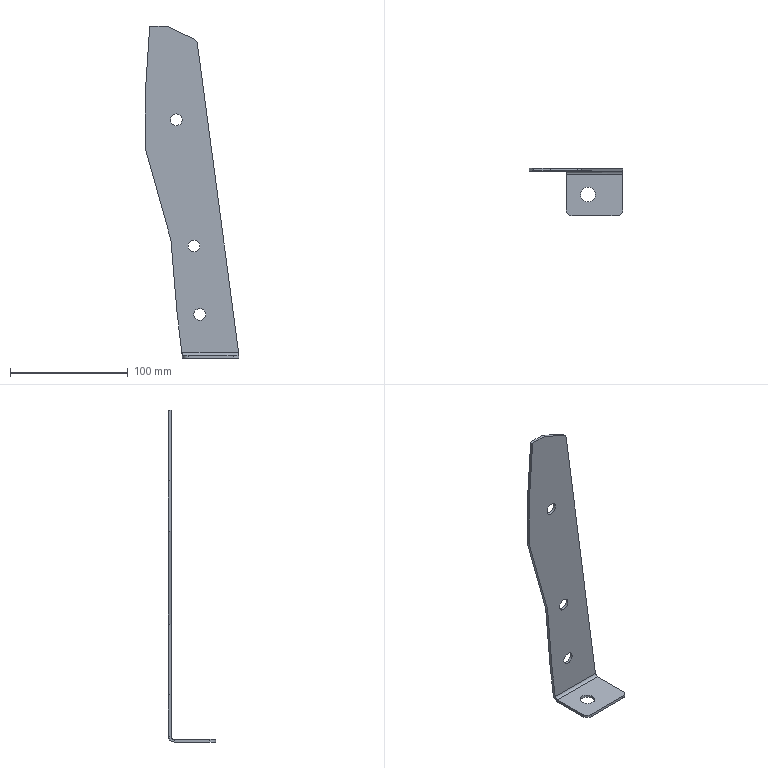Part | SolidWorks | features ICE 2, Fillet 1, FlatPattern 1, SMBaseFlange 1, SheetMetal 1 | 1 solid | 30 faces | box 79.693 x 40 x 281.5 mm | volume 34078 mm3 | plane 15 | cylinder 13 | spline 2 | commonest cylinder face diameters 10 x9 12.5 x2 5 x1 9.6 x1
STEP:
#1=CARTESIAN_POINT('',(3.75,-22.,-279.2));
#2=VERTEX_POINT('',#1);
#3=CARTESIAN_POINT('',(16.25,-22.,-279.2));
#4=VERTEX_POINT('',#3);
#5=CARTESIAN_POINT('',(10.,-22.,-279.2));
#6=DIRECTION('',(0.,0.,1.));
#7=DIRECTION('',(-1.,0.,0.));
#8=AXIS2_PLACEMENT_3D('',#5,#6,#7);
#9=CIRCLE('',#8,6.25);
#10=EDGE_CURVE('',#2,#4,#9,.T.);
#11=ORIENTED_EDGE('',*,*,#10,.T.);
#12=CARTESIAN_POINT('',(16.25,-22.,-281.5));
#13=VERTEX_POINT('',#12);
#14=CARTESIAN_POINT('',(16.25,-22.,0.001));
#15=DIRECTION('',(0.,0.,-1.));
#16=VECTOR('',#15,1000.);
#17=LINE('',#14,#16);
#18=EDGE_CURVE('',#4,#13,#17,.T.);
#19=ORIENTED_EDGE('',*,*,#18,.T.);
#20=CARTESIAN_POINT('',(3.75,-22.,-281.5));
#21=VERTEX_POINT('',#20);
#22=CARTESIAN_POINT('',(10.,-22.,-281.5));
#23=DIRECTION('',(0.,0.,-1.));
#24=DIRECTION('',(-1.,0.,0.));
#25=AXIS2_PLACEMENT_3D('',#22,#23,#24);
#26=CIRCLE('',#25,6.25);
#27=EDGE_CURVE('',#13,#21,#26,.T.);
#28=ORIENTED_EDGE('',*,*,#27,.T.);
#29=CARTESIAN_POINT('',(3.75,-22.,0.001));
#30=DIRECTION('',(0.,0.,-1.));
#31=VECTOR('',#30,1000.);
#32=LINE('',#29,#31);
#33=EDGE_CURVE('',#2,#21,#32,.T.);
#34=ORIENTED_EDGE('',*,*,#33,.F.);
#35=EDGE_LOOP('',(#11,#19,#28,#34));
#36=FACE_OUTER_BOUND('',#35,.T.);
#37=CARTESIAN_POINT('',(10.,-22.,0.001));
#38=DIRECTION('',(0.,0.,-1.));
#39=DIRECTION('',(-1.,0.,0.));
#40=AXIS2_PLACEMENT_3D('',#37,#38,#39);
#41=CYLINDRICAL_SURFACE('',#40,6.25);
#42=ADVANCED_FACE('',(#36),#41,.F.);
#43=CARTESIAN_POINT('',(1.5,-2.3,-191.5));
#44=VERTEX_POINT('',#43);
#45=CARTESIAN_POINT('',(1.5,-2.3,-181.5));
#46=VERTEX_POINT('',#45);
#47=CARTESIAN_POINT('',(1.5,-2.3,-186.5));
#48=DIRECTION('',(0.,1.,0.));
#49=DIRECTION('',(0.,0.,1.));
#50=AXIS2_PLACEMENT_3D('',#47,#48,#49);
#51=CIRCLE('',#50,5.);
#52=EDGE_CURVE('',#44,#46,#51,.T.);
#53=ORIENTED_EDGE('',*,*,#52,.F.);
#54=CARTESIAN_POINT('',(1.5,0.,-191.5));
#55=VERTEX_POINT('',#54);
#56=CARTESIAN_POINT('',(1.5,0.,-191.5));
#57=DIRECTION('',(0.,1.,0.));
#58=VECTOR('',#57,1000.);
#59=LINE('',#56,#58);
#60=EDGE_CURVE('',#44,#55,#59,.T.);
#61=ORIENTED_EDGE('',*,*,#60,.T.);
#62=CARTESIAN_POINT('',(1.5,0.,-181.5));
#63=VERTEX_POINT('',#62);
#64=CARTESIAN_POINT('',(1.5,0.,-186.5));
#65=DIRECTION('',(0.,1.,0.));
#66=DIRECTION('',(0.,0.,1.));
#67=AXIS2_PLACEMENT_3D('',#64,#65,#66);
#68=CIRCLE('',#67,5.);
#69=EDGE_CURVE('',#55,#63,#68,.T.);
#70=ORIENTED_EDGE('',*,*,#69,.T.);
#71=CARTESIAN_POINT('',(1.5,0.,-181.5));
#72=DIRECTION('',(0.,1.,0.));
#73=VECTOR('',#72,1000.);
#74=LINE('',#71,#73);
#75=EDGE_CURVE('',#46,#63,#74,.T.);
#76=ORIENTED_EDGE('',*,*,#75,.F.);
#77=EDGE_LOOP('',(#53,#61,#70,#76));
#78=FACE_OUTER_BOUND('',#77,.T.);
#79=CARTESIAN_POINT('',(1.5,0.,-186.5));
#80=DIRECTION('',(0.,1.,0.));
#81=DIRECTION('',(0.,0.,1.));
#82=AXIS2_PLACEMENT_3D('',#79,#80,#81);
#83=CYLINDRICAL_SURFACE('',#82,5.);
#84=ADVANCED_FACE('',(#78),#83,.F.);
#85=CARTESIAN_POINT('',(-13.5,-2.3,-84.5));
#86=VERTEX_POINT('',#85);
#87=CARTESIAN_POINT('',(-13.5,-2.3,-74.5));
#88=VERTEX_POINT('',#87);
#89=CARTESIAN_POINT('',(-13.5,-2.3,-79.5));
#90=DIRECTION('',(0.,1.,0.));
#91=DIRECTION('',(0.,0.,1.));
#92=AXIS2_PLACEMENT_3D('',#89,#90,#91);
#93=CIRCLE('',#92,5.);
#94=EDGE_CURVE('',#86,#88,#93,.T.);
#95=ORIENTED_EDGE('',*,*,#94,.F.);
#96=CARTESIAN_POINT('',(-13.5,0.,-84.5));
#97=VERTEX_POINT('',#96);
#98=CARTESIAN_POINT('',(-13.5,0.,-84.5));
#99=DIRECTION('',(0.,1.,0.));
#100=VECTOR('',#99,1000.);
#101=LINE('',#98,#100);
#102=EDGE_CURVE('',#86,#97,#101,.T.);
#103=ORIENTED_EDGE('',*,*,#102,.T.);
#104=CARTESIAN_POINT('',(-13.5,0.,-74.5));
#105=VERTEX_POINT('',#104);
#106=CARTESIAN_POINT('',(-13.5,0.,-79.5));
#107=DIRECTION('',(0.,1.,0.));
#108=DIRECTION('',(0.,0.,1.));
#109=AXIS2_PLACEMENT_3D('',#106,#107,#108);
#110=CIRCLE('',#109,5.);
#111=EDGE_CURVE('',#97,#105,#110,.T.);
#112=ORIENTED_EDGE('',*,*,#111,.T.);
#113=CARTESIAN_POINT('',(-13.5,0.,-74.5));
#114=DIRECTION('',(0.,1.,0.));
#115=VECTOR('',#114,1000.);
#116=LINE('',#113,#115);
#117=EDGE_CURVE('',#88,#105,#116,.T.);
#118=ORIENTED_EDGE('',*,*,#117,.F.);
#119=EDGE_LOOP('',(#95,#103,#112,#118));
#120=FACE_OUTER_BOUND('',#119,.T.);
#121=CARTESIAN_POINT('',(-13.5,0.,-79.5));
#122=DIRECTION('',(0.,1.,0.));
#123=DIRECTION('',(0.,0.,1.));
#124=AXIS2_PLACEMENT_3D('',#121,#122,#123);
#125=CYLINDRICAL_SURFACE('',#124,5.);
#126=ADVANCED_FACE('',(#120),#125,.F.);
#127=CARTESIAN_POINT('',(6.5,-2.3,-249.5));
#128=VERTEX_POINT('',#127);
#129=CARTESIAN_POINT('',(6.5,-2.3,-239.5));
#130=VERTEX_POINT('',#129);
#131=CARTESIAN_POINT('',(6.5,-2.3,-244.5));
#132=DIRECTION('',(0.,1.,0.));
#133=DIRECTION('',(0.,0.,1.));
#134=AXIS2_PLACEMENT_3D('',#131,#132,#133);
#135=CIRCLE('',#134,5.);
#136=EDGE_CURVE('',#128,#130,#135,.T.);
#137=ORIENTED_EDGE('',*,*,#136,.F.);
#138=CARTESIAN_POINT('',(6.5,0.,-249.5));
#139=VERTEX_POINT('',#138);
#140=CARTESIAN_POINT('',(6.5,0.,-249.5));
#141=DIRECTION('',(0.,1.,0.));
#142=VECTOR('',#141,1000.);
#143=LINE('',#140,#142);
#144=EDGE_CURVE('',#128,#139,#143,.T.);
#145=ORIENTED_EDGE('',*,*,#144,.T.);
#146=CARTESIAN_POINT('',(6.5,0.,-239.5));
#147=VERTEX_POINT('',#146);
#148=CARTESIAN_POINT('',(6.5,0.,-244.5));
#149=DIRECTION('',(0.,1.,0.));
#150=DIRECTION('',(0.,0.,1.));
#151=AXIS2_PLACEMENT_3D('',#148,#149,#150);
#152=CIRCLE('',#151,5.);
#153=EDGE_CURVE('',#139,#147,#152,.T.);
#154=ORIENTED_EDGE('',*,*,#153,.T.);
#155=CARTESIAN_POINT('',(6.5,0.,-239.5));
#156=DIRECTION('',(0.,1.,0.));
#157=VECTOR('',#156,1000.);
#158=LINE('',#155,#157);
#159=EDGE_CURVE('',#130,#147,#158,.T.);
#160=ORIENTED_EDGE('',*,*,#159,.F.);
#161=EDGE_LOOP('',(#137,#145,#154,#160));
#162=FACE_OUTER_BOUND('',#161,.T.);
#163=CARTESIAN_POINT('',(6.5,0.,-244.5));
#164=DIRECTION('',(0.,1.,0.));
#165=DIRECTION('',(0.,0.,1.));
#166=AXIS2_PLACEMENT_3D('',#163,#164,#165);
#167=CYLINDRICAL_SURFACE('',#166,5.);
#168=ADVANCED_FACE('',(#162),#167,.F.);
#169=CARTESIAN_POINT('',(-40.,0.,-60.));
#170=VERTEX_POINT('',#169);
#171=CARTESIAN_POINT('',(-40.,0.,-103.));
#172=VERTEX_POINT('',#171);
#173=CARTESIAN_POINT('',(-40.,0.,0.));
#174=DIRECTION('',(0.,0.,-1.));
#175=VECTOR('',#174,1000.);
#176=LINE('',#173,#175);
#177=EDGE_CURVE('',#170,#172,#176,.T.);
#178=ORIENTED_EDGE('',*,*,#177,.T.);
#179=CARTESIAN_POINT('',(-40.,-2.3,-103.));
#180=VERTEX_POINT('',#179);
#181=CARTESIAN_POINT('',(-40.,0.,-103.));
#182=DIRECTION('',(0.,-1.,0.));
#183=VECTOR('',#182,1000.);
#184=LINE('',#181,#183);
#185=EDGE_CURVE('',#172,#180,#184,.T.);
#186=ORIENTED_EDGE('',*,*,#185,.T.);
#187=CARTESIAN_POINT('',(-40.,-2.3,-60.));
#188=VERTEX_POINT('',#187);
#189=CARTESIAN_POINT('',(-40.,-2.3,0.));
#190=DIRECTION('',(0.,0.,-1.));
#191=VECTOR('',#190,1000.);
#192=LINE('',#189,#191);
#193=EDGE_CURVE('',#188,#180,#192,.T.);
#194=ORIENTED_EDGE('',*,*,#193,.F.);
#195=CARTESIAN_POINT('',(-40.,-2.3,-60.));
#196=DIRECTION('',(0.,1.,0.));
#197=VECTOR('',#196,1000.);
#198=LINE('',#195,#197);
#199=EDGE_CURVE('',#188,#170,#198,.T.);
#200=ORIENTED_EDGE('',*,*,#199,.T.);
#201=EDGE_LOOP('',(#178,#186,#194,#200));
#202=FACE_OUTER_BOUND('',#201,.T.);
#203=CARTESIAN_POINT('',(-40.,-4.8,-279.2));
#204=DIRECTION('',(-1.,0.,0.));
#205=DIRECTION('',(0.,0.,1.));
#206=AXIS2_PLACEMENT_3D('',#203,#204,#205);
#207=PLANE('',#206);
#208=ADVANCED_FACE('',(#202),#207,.T.);
#209=ORIENTED_EDGE('',*,*,#10,.F.);
#210=CARTESIAN_POINT('',(10.,-22.,-279.2));
#211=DIRECTION('',(0.,0.,1.));
#212=DIRECTION('',(-1.,0.,0.));
#213=AXIS2_PLACEMENT_3D('',#210,#211,#212);
#214=CIRCLE('',#213,6.25);
#215=EDGE_CURVE('',#4,#2,#214,.T.);
#216=ORIENTED_EDGE('',*,*,#215,.F.);
#217=EDGE_LOOP('',(#209,#216));
#218=FACE_BOUND('',#217,.T.);
#219=CARTESIAN_POINT('',(34.693,-40.,-279.2));
#220=VERTEX_POINT('',#219);
#221=CARTESIAN_POINT('',(-3.3,-40.,-279.2));
#222=VERTEX_POINT('',#221);
#223=CARTESIAN_POINT('',(40.,-40.,-279.2));
#224=DIRECTION('',(-1.,0.,0.));
#225=VECTOR('',#224,1000.);
#226=LINE('',#223,#225);
#227=EDGE_CURVE('',#220,#222,#226,.T.);
#228=ORIENTED_EDGE('',*,*,#227,.F.);
#229=CARTESIAN_POINT('',(39.693,-35.,-279.2));
#230=VERTEX_POINT('',#229);
#231=CARTESIAN_POINT('',(34.693,-35.,-279.2));
#232=DIRECTION('',(0.,0.,1.));
#233=DIRECTION('',(-1.,0.,0.));
#234=AXIS2_PLACEMENT_3D('',#231,#232,#233);
#235=CIRCLE('',#234,5.);
#236=EDGE_CURVE('',#220,#230,#235,.T.);
#237=ORIENTED_EDGE('',*,*,#236,.T.);
#238=CARTESIAN_POINT('',(39.693,-4.8,-279.2));
#239=VERTEX_POINT('',#238);
#240=CARTESIAN_POINT('',(39.693,0.,-279.2));
#241=DIRECTION('',(0.,1.,0.));
#242=VECTOR('',#241,1000.);
#243=LINE('',#240,#242);
#244=EDGE_CURVE('',#230,#239,#243,.T.);
#245=ORIENTED_EDGE('',*,*,#244,.T.);
#246=CARTESIAN_POINT('',(-8.3,-4.8,-279.2));
#247=VERTEX_POINT('',#246);
#248=CARTESIAN_POINT('',(40.,-4.8,-279.2));
#249=DIRECTION('',(-1.,0.,0.));
#250=VECTOR('',#249,1000.);
#251=LINE('',#248,#250);
#252=EDGE_CURVE('',#239,#247,#251,.T.);
#253=ORIENTED_EDGE('',*,*,#252,.T.);
#254=CARTESIAN_POINT('',(-8.3,-35.,-279.2));
#255=VERTEX_POINT('',#254);
#256=CARTESIAN_POINT('',(-8.3,0.,-279.2));
#257=DIRECTION('',(0.,1.,0.));
#258=VECTOR('',#257,1000.);
#259=LINE('',#256,#258);
#260=EDGE_CURVE('',#255,#247,#259,.T.);
#261=ORIENTED_EDGE('',*,*,#260,.F.);
#262=CARTESIAN_POINT('',(-3.3,-35.,-279.2));
#263=DIRECTION('',(0.,0.,1.));
#264=DIRECTION('',(-1.,0.,0.));
#265=AXIS2_PLACEMENT_3D('',#262,#263,#264);
#266=CIRCLE('',#265,5.);
#267=EDGE_CURVE('',#255,#222,#266,.T.);
#268=ORIENTED_EDGE('',*,*,#267,.T.);
#269=EDGE_LOOP('',(#228,#237,#245,#253,#261,#268));
#270=FACE_OUTER_BOUND('',#269,.T.);
#271=CARTESIAN_POINT('',(40.,0.,-279.2));
#272=DIRECTION('',(0.,0.,-1.));
#273=DIRECTION('',(-1.,0.,0.));
#274=AXIS2_PLACEMENT_3D('',#271,#272,#273);
#275=PLANE('',#274);
#276=ADVANCED_FACE('',(#218,#270),#275,.F.);
#277=CARTESIAN_POINT('',(34.693,-40.,-281.5));
#278=VERTEX_POINT('',#277);
#279=CARTESIAN_POINT('',(-3.3,-40.,-281.5));
#280=VERTEX_POINT('',#279);
#281=CARTESIAN_POINT('',(40.,-40.,-281.5));
#282=DIRECTION('',(-1.,0.,0.));
#283=VECTOR('',#282,1000.);
#284=LINE('',#281,#283);
#285=EDGE_CURVE('',#278,#280,#284,.T.);
#286=ORIENTED_EDGE('',*,*,#285,.F.);
#287=CARTESIAN_POINT('',(34.693,-40.,-281.5));
#288=DIRECTION('',(0.,0.,1.));
#289=VECTOR('',#288,1000.);
#290=LINE('',#287,#289);
#291=EDGE_CURVE('',#278,#220,#290,.T.);
#292=ORIENTED_EDGE('',*,*,#291,.T.);
#293=ORIENTED_EDGE('',*,*,#227,.T.);
#294=CARTESIAN_POINT('',(-3.3,-40.,-281.5));
#295=DIRECTION('',(0.,0.,-1.));
#296=VECTOR('',#295,1000.);
#297=LINE('',#294,#296);
#298=EDGE_CURVE('',#222,#280,#297,.T.);
#299=ORIENTED_EDGE('',*,*,#298,.T.);
#300=EDGE_LOOP('',(#286,#292,#293,#299));
#301=FACE_OUTER_BOUND('',#300,.T.);
#302=CARTESIAN_POINT('',(40.,-40.,-281.5));
#303=DIRECTION('',(0.,-1.,0.));
#304=DIRECTION('',(0.,0.,-1.));
#305=AXIS2_PLACEMENT_3D('',#302,#303,#304);
#306=PLANE('',#305);
#307=ADVANCED_FACE('',(#301),#306,.T.);
#308=CARTESIAN_POINT('',(10.,-22.,-281.5));
#309=DIRECTION('',(0.,0.,-1.));
#310=DIRECTION('',(-1.,0.,0.));
#311=AXIS2_PLACEMENT_3D('',#308,#309,#310);
#312=CIRCLE('',#311,6.25);
#313=EDGE_CURVE('',#21,#13,#312,.T.);
#314=ORIENTED_EDGE('',*,*,#313,.F.);
#315=ORIENTED_EDGE('',*,*,#27,.F.);
#316=EDGE_LOOP('',(#314,#315));
#317=FACE_BOUND('',#316,.T.);
#318=CARTESIAN_POINT('',(39.693,-35.,-281.5));
#319=VERTEX_POINT('',#318);
#320=CARTESIAN_POINT('',(39.693,-4.8,-281.5));
#321=VERTEX_POINT('',#320);
#322=CARTESIAN_POINT('',(39.693,0.,-281.5));
#323=DIRECTION('',(0.,1.,0.));
#324=VECTOR('',#323,1000.);
#325=LINE('',#322,#324);
#326=EDGE_CURVE('',#319,#321,#325,.T.);
#327=ORIENTED_EDGE('',*,*,#326,.F.);
#328=CARTESIAN_POINT('',(34.693,-35.,-281.5));
#329=DIRECTION('',(0.,0.,-1.));
#330=DIRECTION('',(-1.,0.,0.));
#331=AXIS2_PLACEMENT_3D('',#328,#329,#330);
#332=CIRCLE('',#331,5.);
#333=EDGE_CURVE('',#319,#278,#332,.T.);
#334=ORIENTED_EDGE('',*,*,#333,.T.);
#335=ORIENTED_EDGE('',*,*,#285,.T.);
#336=CARTESIAN_POINT('',(-8.3,-35.,-281.5));
#337=VERTEX_POINT('',#336);
#338=CARTESIAN_POINT('',(-3.3,-35.,-281.5));
#339=DIRECTION('',(0.,0.,-1.));
#340=DIRECTION('',(-1.,0.,0.));
#341=AXIS2_PLACEMENT_3D('',#338,#339,#340);
#342=CIRCLE('',#341,5.);
#343=EDGE_CURVE('',#280,#337,#342,.T.);
#344=ORIENTED_EDGE('',*,*,#343,.T.);
#345=CARTESIAN_POINT('',(-8.3,-4.8,-281.5));
#346=VERTEX_POINT('',#345);
#347=CARTESIAN_POINT('',(-8.3,-40.,-281.5));
#348=DIRECTION('',(0.,1.,0.));
#349=VECTOR('',#348,1000.);
#350=LINE('',#347,#349);
#351=EDGE_CURVE('',#337,#346,#350,.T.);
#352=ORIENTED_EDGE('',*,*,#351,.T.);
#353=CARTESIAN_POINT('',(40.,-4.8,-281.5));
#354=DIRECTION('',(-1.,0.,0.));
#355=VECTOR('',#354,1000.);
#356=LINE('',#353,#355);
#357=EDGE_CURVE('',#321,#346,#356,.T.);
#358=ORIENTED_EDGE('',*,*,#357,.F.);
#359=EDGE_LOOP('',(#327,#334,#335,#344,#352,#358));
#360=FACE_OUTER_BOUND('',#359,.T.);
#361=CARTESIAN_POINT('',(40.,0.,-281.5));
#362=DIRECTION('',(0.,0.,-1.));
#363=DIRECTION('',(-1.,0.,0.));
#364=AXIS2_PLACEMENT_3D('',#361,#362,#363);
#365=PLANE('',#364);
#366=ADVANCED_FACE('',(#317,#360),#365,.T.);
#367=ORIENTED_EDGE('',*,*,#357,.T.);
#368=CARTESIAN_POINT('',(-8.864,0.,-276.7));
#369=VERTEX_POINT('',#368);
#370=CARTESIAN_POINT('',(-8.864,0.,-276.7));
#371=CARTESIAN_POINT('',(-8.534,0.,-279.512));
#372=CARTESIAN_POINT('',(-8.3,-1.988,-281.5));
#373=CARTESIAN_POINT('',(-8.3,-4.8,-281.5));
#374=(BOUNDED_CURVE()B_SPLINE_CURVE(3,(#370,#371,#372,#373),.UNSPECIFIED.,.F.,.F.)B_SPLINE_CURVE_WITH_KNOTS((4,4),(1.571,3.142),.UNSPECIFIED.)CURVE()GEOMETRIC_REPRESENTATION_ITEM()RATIONAL_B_SPLINE_CURVE((1.,0.8047,0.8047,1.))REPRESENTATION_ITEM(''));
#375=EDGE_CURVE('',#369,#346,#374,.T.);
#376=ORIENTED_EDGE('',*,*,#375,.F.);
#377=CARTESIAN_POINT('',(39.359,0.,-276.7));
#378=VERTEX_POINT('',#377);
#379=CARTESIAN_POINT('',(40.,0.,-276.7));
#380=DIRECTION('',(-1.,0.,0.));
#381=VECTOR('',#380,1000.);
#382=LINE('',#379,#381);
#383=EDGE_CURVE('',#378,#369,#382,.T.);
#384=ORIENTED_EDGE('',*,*,#383,.F.);
#385=CARTESIAN_POINT('',(39.693,-4.8,-281.5));
#386=CARTESIAN_POINT('',(39.693,-1.988,-281.5));
#387=CARTESIAN_POINT('',(39.554,0.,-279.512));
#388=CARTESIAN_POINT('',(39.359,0.,-276.7));
#389=(BOUNDED_CURVE()B_SPLINE_CURVE(3,(#385,#386,#387,#388),.UNSPECIFIED.,.F.,.F.)B_SPLINE_CURVE_WITH_KNOTS((4,4),(3.142,4.712),.UNSPECIFIED.)CURVE()GEOMETRIC_REPRESENTATION_ITEM()RATIONAL_B_SPLINE_CURVE((1.,0.8047,0.8047,1.))REPRESENTATION_ITEM(''));
#390=EDGE_CURVE('',#321,#378,#389,.T.);
#391=ORIENTED_EDGE('',*,*,#390,.F.);
#392=EDGE_LOOP('',(#367,#376,#384,#391));
#393=FACE_OUTER_BOUND('',#392,.T.);
#394=CARTESIAN_POINT('',(40.,-4.8,-276.7));
#395=DIRECTION('',(-1.,0.,0.));
#396=DIRECTION('',(0.,0.,1.));
#397=AXIS2_PLACEMENT_3D('',#394,#395,#396);
#398=CYLINDRICAL_SURFACE('',#397,4.8);
#399=ADVANCED_FACE('',(#393),#398,.T.);
#400=CARTESIAN_POINT('',(-22.,-2.3,0.));
#401=VERTEX_POINT('',#400);
#402=CARTESIAN_POINT('',(-36.,-2.3,0.));
#403=VERTEX_POINT('',#402);
#404=CARTESIAN_POINT('',(40.,-2.3,0.));
#405=DIRECTION('',(-1.,0.,0.));
#406=VECTOR('',#405,1000.);
#407=LINE('',#404,#406);
#408=EDGE_CURVE('',#401,#403,#407,.T.);
#409=ORIENTED_EDGE('',*,*,#408,.F.);
#410=CARTESIAN_POINT('',(-22.,0.,0.));
#411=VERTEX_POINT('',#410);
#412=CARTESIAN_POINT('',(-22.,-2.3,0.));
#413=DIRECTION('',(0.,1.,0.));
#414=VECTOR('',#413,1000.);
#415=LINE('',#412,#414);
#416=EDGE_CURVE('',#401,#411,#415,.T.);
#417=ORIENTED_EDGE('',*,*,#416,.T.);
#418=CARTESIAN_POINT('',(-36.,0.,0.));
#419=VERTEX_POINT('',#418);
#420=CARTESIAN_POINT('',(40.,0.,0.));
#421=DIRECTION('',(-1.,0.,0.));
#422=VECTOR('',#421,1000.);
#423=LINE('',#420,#422);
#424=EDGE_CURVE('',#411,#419,#423,.T.);
#425=ORIENTED_EDGE('',*,*,#424,.T.);
#426=CARTESIAN_POINT('',(-36.,-2.3,0.));
#427=DIRECTION('',(0.,1.,0.));
#428=VECTOR('',#427,1000.);
#429=LINE('',#426,#428);
#430=EDGE_CURVE('',#403,#419,#429,.T.);
#431=ORIENTED_EDGE('',*,*,#430,.F.);
#432=EDGE_LOOP('',(#409,#417,#425,#431));
#433=FACE_OUTER_BOUND('',#432,.T.);
#434=CARTESIAN_POINT('',(40.,-2.3,0.));
#435=DIRECTION('',(0.,0.,1.));
#436=DIRECTION('',(1.,0.,0.));
#437=AXIS2_PLACEMENT_3D('',#434,#435,#436);
#438=PLANE('',#437);
#439=ADVANCED_FACE('',(#433),#438,.T.);
#440=CARTESIAN_POINT('',(-8.864,-2.3,-276.7));
#441=VERTEX_POINT('',#440);
#442=CARTESIAN_POINT('',(-8.864,-2.3,-276.7));
#443=CARTESIAN_POINT('',(-8.534,-2.3,-278.164));
#444=CARTESIAN_POINT('',(-8.3,-3.336,-279.2));
#445=CARTESIAN_POINT('',(-8.3,-4.8,-279.2));
#446=(BOUNDED_CURVE()B_SPLINE_CURVE(3,(#442,#443,#444,#445),.UNSPECIFIED.,.F.,.F.)B_SPLINE_CURVE_WITH_KNOTS((4,4),(1.571,3.142),.UNSPECIFIED.)CURVE()GEOMETRIC_REPRESENTATION_ITEM()RATIONAL_B_SPLINE_CURVE((1.,0.8047,0.8047,1.))REPRESENTATION_ITEM(''));
#447=EDGE_CURVE('',#441,#247,#446,.T.);
#448=ORIENTED_EDGE('',*,*,#447,.T.);
#449=ORIENTED_EDGE('',*,*,#252,.F.);
#450=CARTESIAN_POINT('',(39.359,-2.3,-276.7));
#451=VERTEX_POINT('',#450);
#452=CARTESIAN_POINT('',(39.693,-4.8,-279.2));
#453=CARTESIAN_POINT('',(39.693,-3.336,-279.2));
#454=CARTESIAN_POINT('',(39.554,-2.3,-278.164));
#455=CARTESIAN_POINT('',(39.359,-2.3,-276.7));
#456=(BOUNDED_CURVE()B_SPLINE_CURVE(3,(#452,#453,#454,#455),.UNSPECIFIED.,.F.,.T.)B_SPLINE_CURVE_WITH_KNOTS((4,4),(3.142,4.712),.UNSPECIFIED.)CURVE()GEOMETRIC_REPRESENTATION_ITEM()RATIONAL_B_SPLINE_CURVE((1.,0.8047,0.8047,1.))REPRESENTATION_ITEM(''));
#457=EDGE_CURVE('',#239,#451,#456,.T.);
#458=ORIENTED_EDGE('',*,*,#457,.T.);
#459=CARTESIAN_POINT('',(40.,-2.3,-276.7));
#460=DIRECTION('',(-1.,0.,0.));
#461=VECTOR('',#460,1000.);
#462=LINE('',#459,#461);
#463=EDGE_CURVE('',#451,#441,#462,.T.);
#464=ORIENTED_EDGE('',*,*,#463,.T.);
#465=EDGE_LOOP('',(#448,#449,#458,#464));
#466=FACE_OUTER_BOUND('',#465,.T.);
#467=CARTESIAN_POINT('',(40.,-4.8,-276.7));
#468=DIRECTION('',(-1.,0.,0.));
#469=DIRECTION('',(0.,0.,1.));
#470=AXIS2_PLACEMENT_3D('',#467,#468,#469);
#471=CYLINDRICAL_SURFACE('',#470,2.5);
#472=ADVANCED_FACE('',(#466),#471,.F.);
#473=CARTESIAN_POINT('',(1.5,0.,-186.5));
#474=DIRECTION('',(0.,1.,0.));
#475=DIRECTION('',(0.,0.,1.));
#476=AXIS2_PLACEMENT_3D('',#473,#474,#475);
#477=CIRCLE('',#476,5.);
#478=EDGE_CURVE('',#63,#55,#477,.T.);
#479=ORIENTED_EDGE('',*,*,#478,.F.);
#480=ORIENTED_EDGE('',*,*,#69,.F.);
#481=EDGE_LOOP('',(#479,#480));
#482=FACE_BOUND('',#481,.T.);
#483=CARTESIAN_POINT('',(-13.5,0.,-79.5));
#484=DIRECTION('',(0.,1.,0.));
#485=DIRECTION('',(0.,0.,1.));
#486=AXIS2_PLACEMENT_3D('',#483,#484,#485);
#487=CIRCLE('',#486,5.);
#488=EDGE_CURVE('',#105,#97,#487,.T.);
#489=ORIENTED_EDGE('',*,*,#488,.F.);
#490=ORIENTED_EDGE('',*,*,#111,.F.);
#491=EDGE_LOOP('',(#489,#490));
#492=FACE_BOUND('',#491,.T.);
#493=CARTESIAN_POINT('',(6.5,0.,-244.5));
#494=DIRECTION('',(0.,1.,0.));
#495=DIRECTION('',(0.,0.,1.));
#496=AXIS2_PLACEMENT_3D('',#493,#494,#495);
#497=CIRCLE('',#496,5.);
#498=EDGE_CURVE('',#147,#139,#497,.T.);
#499=ORIENTED_EDGE('',*,*,#498,.F.);
#500=ORIENTED_EDGE('',*,*,#153,.F.);
#501=EDGE_LOOP('',(#499,#500));
#502=FACE_BOUND('',#501,.T.);
#503=ORIENTED_EDGE('',*,*,#383,.T.);
#504=CARTESIAN_POINT('',(-13.,0.,-241.5));
#505=VERTEX_POINT('',#504);
#506=CARTESIAN_POINT('',(-13.,0.,-241.5));
#507=DIRECTION('',(0.1167,0.,-0.9932));
#508=VECTOR('',#507,1000.);
#509=LINE('',#506,#508);
#510=EDGE_CURVE('',#505,#369,#509,.T.);
#511=ORIENTED_EDGE('',*,*,#510,.F.);
#512=CARTESIAN_POINT('',(-18.,0.,-181.5));
#513=VERTEX_POINT('',#512);
#514=CARTESIAN_POINT('',(-18.,0.,-181.5));
#515=DIRECTION('',(0.08305,0.,-0.9965));
#516=VECTOR('',#515,1000.);
#517=LINE('',#514,#516);
#518=EDGE_CURVE('',#513,#505,#517,.T.);
#519=ORIENTED_EDGE('',*,*,#518,.F.);
#520=CARTESIAN_POINT('',(-40.,0.,-103.));
#521=DIRECTION('',(0.2699,0.,-0.9629));
#522=VECTOR('',#521,1000.);
#523=LINE('',#520,#522);
#524=EDGE_CURVE('',#172,#513,#523,.T.);
#525=ORIENTED_EDGE('',*,*,#524,.F.);
#526=ORIENTED_EDGE('',*,*,#177,.F.);
#527=CARTESIAN_POINT('',(-35.664,0.,5.044));
#528=DIRECTION('',(-0.06652,0.,-0.9978));
#529=VECTOR('',#528,1000.);
#530=LINE('',#527,#529);
#531=EDGE_CURVE('',#419,#170,#530,.T.);
#532=ORIENTED_EDGE('',*,*,#531,.F.);
#533=ORIENTED_EDGE('',*,*,#424,.F.);
#534=CARTESIAN_POINT('',(1.503,0.,-10.848));
#535=VERTEX_POINT('',#534);
#536=CARTESIAN_POINT('',(29.112,0.,-23.59));
#537=DIRECTION('',(-0.908,0.,0.4191));
#538=VECTOR('',#537,1000.);
#539=LINE('',#536,#538);
#540=EDGE_CURVE('',#535,#411,#539,.T.);
#541=ORIENTED_EDGE('',*,*,#540,.F.);
#542=CARTESIAN_POINT('',(4.364,0.,-14.725));
#543=VERTEX_POINT('',#542);
#544=CARTESIAN_POINT('',(-0.5919,0.,-15.388));
#545=DIRECTION('',(0.,-1.,0.));
#546=DIRECTION('',(0.,0.,1.));
#547=AXIS2_PLACEMENT_3D('',#544,#545,#546);
#548=CIRCLE('',#547,5.);
#549=EDGE_CURVE('',#543,#535,#548,.T.);
#550=ORIENTED_EDGE('',*,*,#549,.F.);
#551=CARTESIAN_POINT('',(3.056,0.,-4.935));
#552=DIRECTION('',(-0.1324,0.,0.9912));
#553=VECTOR('',#552,1000.);
#554=LINE('',#551,#553);
#555=EDGE_CURVE('',#378,#543,#554,.T.);
#556=ORIENTED_EDGE('',*,*,#555,.F.);
#557=EDGE_LOOP('',(#503,#511,#519,#525,#526,#532,#533,#541,#550,#556));
#558=FACE_OUTER_BOUND('',#557,.T.);
#559=CARTESIAN_POINT('',(40.,0.,0.));
#560=DIRECTION('',(0.,1.,0.));
#561=DIRECTION('',(0.,0.,1.));
#562=AXIS2_PLACEMENT_3D('',#559,#560,#561);
#563=PLANE('',#562);
#564=ADVANCED_FACE('',(#482,#492,#502,#558),#563,.T.);
#565=CARTESIAN_POINT('',(-13.,-2.3,-241.5));
#566=VERTEX_POINT('',#565);
#567=CARTESIAN_POINT('',(-13.,-2.3,-241.5));
#568=DIRECTION('',(0.1167,0.,-0.9932));
#569=VECTOR('',#568,1000.);
#570=LINE('',#567,#569);
#571=EDGE_CURVE('',#566,#441,#570,.T.);
#572=ORIENTED_EDGE('',*,*,#571,.T.);
#573=ORIENTED_EDGE('',*,*,#463,.F.);
#574=CARTESIAN_POINT('',(4.364,-2.3,-14.725));
#575=VERTEX_POINT('',#574);
#576=CARTESIAN_POINT('',(3.056,-2.3,-4.935));
#577=DIRECTION('',(-0.1324,0.,0.9912));
#578=VECTOR('',#577,1000.);
#579=LINE('',#576,#578);
#580=EDGE_CURVE('',#451,#575,#579,.T.);
#581=ORIENTED_EDGE('',*,*,#580,.T.);
#582=CARTESIAN_POINT('',(1.503,-2.3,-10.848));
#583=VERTEX_POINT('',#582);
#584=CARTESIAN_POINT('',(-0.5919,-2.3,-15.388));
#585=DIRECTION('',(0.,-1.,0.));
#586=DIRECTION('',(0.,0.,1.));
#587=AXIS2_PLACEMENT_3D('',#584,#585,#586);
#588=CIRCLE('',#587,5.);
#589=EDGE_CURVE('',#575,#583,#588,.T.);
#590=ORIENTED_EDGE('',*,*,#589,.T.);
#591=CARTESIAN_POINT('',(29.112,-2.3,-23.59));
#592=DIRECTION('',(-0.908,0.,0.4191));
#593=VECTOR('',#592,1000.);
#594=LINE('',#591,#593);
#595=EDGE_CURVE('',#583,#401,#594,.T.);
#596=ORIENTED_EDGE('',*,*,#595,.T.);
#597=ORIENTED_EDGE('',*,*,#408,.T.);
#598=CARTESIAN_POINT('',(-35.664,-2.3,5.044));
#599=DIRECTION('',(-0.06652,0.,-0.9978));
#600=VECTOR('',#599,1000.);
#601=LINE('',#598,#600);
#602=EDGE_CURVE('',#403,#188,#601,.T.);
#603=ORIENTED_EDGE('',*,*,#602,.T.);
#604=ORIENTED_EDGE('',*,*,#193,.T.);
#605=CARTESIAN_POINT('',(-18.,-2.3,-181.5));
#606=VERTEX_POINT('',#605);
#607=CARTESIAN_POINT('',(-40.,-2.3,-103.));
#608=DIRECTION('',(0.2699,0.,-0.9629));
#609=VECTOR('',#608,1000.);
#610=LINE('',#607,#609);
#611=EDGE_CURVE('',#180,#606,#610,.T.);
#612=ORIENTED_EDGE('',*,*,#611,.T.);
#613=CARTESIAN_POINT('',(-18.,-2.3,-181.5));
#614=DIRECTION('',(0.08305,0.,-0.9965));
#615=VECTOR('',#614,1000.);
#616=LINE('',#613,#615);
#617=EDGE_CURVE('',#606,#566,#616,.T.);
#618=ORIENTED_EDGE('',*,*,#617,.T.);
#619=EDGE_LOOP('',(#572,#573,#581,#590,#596,#597,#603,#604,#612,#618));
#620=FACE_OUTER_BOUND('',#619,.T.);
#621=CARTESIAN_POINT('',(1.5,-2.3,-186.5));
#622=DIRECTION('',(0.,1.,0.));
#623=DIRECTION('',(0.,0.,1.));
#624=AXIS2_PLACEMENT_3D('',#621,#622,#623);
#625=CIRCLE('',#624,5.);
#626=EDGE_CURVE('',#46,#44,#625,.T.);
#627=ORIENTED_EDGE('',*,*,#626,.T.);
#628=ORIENTED_EDGE('',*,*,#52,.T.);
#629=EDGE_LOOP('',(#627,#628));
#630=FACE_BOUND('',#629,.T.);
#631=CARTESIAN_POINT('',(-13.5,-2.3,-79.5));
#632=DIRECTION('',(0.,1.,0.));
#633=DIRECTION('',(0.,0.,1.));
#634=AXIS2_PLACEMENT_3D('',#631,#632,#633);
#635=CIRCLE('',#634,5.);
#636=EDGE_CURVE('',#88,#86,#635,.T.);
#637=ORIENTED_EDGE('',*,*,#636,.T.);
#638=ORIENTED_EDGE('',*,*,#94,.T.);
#639=EDGE_LOOP('',(#637,#638));
#640=FACE_BOUND('',#639,.T.);
#641=CARTESIAN_POINT('',(6.5,-2.3,-244.5));
#642=DIRECTION('',(0.,1.,0.));
#643=DIRECTION('',(0.,0.,1.));
#644=AXIS2_PLACEMENT_3D('',#641,#642,#643);
#645=CIRCLE('',#644,5.);
#646=EDGE_CURVE('',#130,#128,#645,.T.);
#647=ORIENTED_EDGE('',*,*,#646,.T.);
#648=ORIENTED_EDGE('',*,*,#136,.T.);
#649=EDGE_LOOP('',(#647,#648));
#650=FACE_BOUND('',#649,.T.);
#651=CARTESIAN_POINT('',(40.,-2.3,0.));
#652=DIRECTION('',(0.,1.,0.));
#653=DIRECTION('',(0.,0.,1.));
#654=AXIS2_PLACEMENT_3D('',#651,#652,#653);
#655=PLANE('',#654);
#656=ADVANCED_FACE('',(#620,#630,#640,#650),#655,.F.);
#657=ORIENTED_EDGE('',*,*,#244,.F.);
#658=CARTESIAN_POINT('',(39.693,-35.,-279.2));
#659=DIRECTION('',(0.,0.,-1.));
#660=VECTOR('',#659,1000.);
#661=LINE('',#658,#660);
#662=EDGE_CURVE('',#230,#319,#661,.T.);
#663=ORIENTED_EDGE('',*,*,#662,.T.);
#664=ORIENTED_EDGE('',*,*,#326,.T.);
#665=CARTESIAN_POINT('',(39.693,-4.8,-279.2));
#666=DIRECTION('',(0.,0.,-1.));
#667=VECTOR('',#666,1000.);
#668=LINE('',#665,#667);
#669=EDGE_CURVE('',#239,#321,#668,.T.);
#670=ORIENTED_EDGE('',*,*,#669,.F.);
#671=EDGE_LOOP('',(#657,#663,#664,#670));
#672=FACE_OUTER_BOUND('',#671,.T.);
#673=CARTESIAN_POINT('',(39.693,0.,-279.2));
#674=DIRECTION('',(-1.,0.,0.));
#675=DIRECTION('',(0.,1.,0.));
#676=AXIS2_PLACEMENT_3D('',#673,#674,#675);
#677=PLANE('',#676);
#678=ADVANCED_FACE('',(#672),#677,.F.);
#679=CARTESIAN_POINT('',(4.364,-2.3,-14.725));
#680=DIRECTION('',(0.,1.,0.));
#681=VECTOR('',#680,1000.);
#682=LINE('',#679,#681);
#683=EDGE_CURVE('',#575,#543,#682,.T.);
#684=ORIENTED_EDGE('',*,*,#683,.F.);
#685=ORIENTED_EDGE('',*,*,#580,.F.);
#686=CARTESIAN_POINT('',(39.359,-2.3,-276.7));
#687=DIRECTION('',(0.,1.,0.));
#688=VECTOR('',#687,1000.);
#689=LINE('',#686,#688);
#690=EDGE_CURVE('',#451,#378,#689,.T.);
#691=ORIENTED_EDGE('',*,*,#690,.T.);
#692=ORIENTED_EDGE('',*,*,#555,.T.);
#693=EDGE_LOOP('',(#684,#685,#691,#692));
#694=FACE_OUTER_BOUND('',#693,.T.);
#695=CARTESIAN_POINT('',(3.056,-2.3,-4.935));
#696=DIRECTION('',(-0.9912,0.,-0.1324));
#697=DIRECTION('',(-0.1324,0.,0.9912));
#698=AXIS2_PLACEMENT_3D('',#695,#696,#697);
#699=PLANE('',#698);
#700=ADVANCED_FACE('',(#694),#699,.F.);
#701=ORIENTED_EDGE('',*,*,#416,.F.);
#702=ORIENTED_EDGE('',*,*,#595,.F.);
#703=CARTESIAN_POINT('',(1.503,-2.3,-10.848));
#704=DIRECTION('',(0.,1.,0.));
#705=VECTOR('',#704,1000.);
#706=LINE('',#703,#705);
#707=EDGE_CURVE('',#583,#535,#706,.T.);
#708=ORIENTED_EDGE('',*,*,#707,.T.);
#709=ORIENTED_EDGE('',*,*,#540,.T.);
#710=EDGE_LOOP('',(#701,#702,#708,#709));
#711=FACE_OUTER_BOUND('',#710,.T.);
#712=CARTESIAN_POINT('',(29.112,-2.3,-23.59));
#713=DIRECTION('',(-0.4191,0.,-0.908));
#714=DIRECTION('',(-0.908,0.,0.4191));
#715=AXIS2_PLACEMENT_3D('',#712,#713,#714);
#716=PLANE('',#715);
#717=ADVANCED_FACE('',(#711),#716,.F.);
#718=ORIENTED_EDGE('',*,*,#589,.F.);
#719=ORIENTED_EDGE('',*,*,#683,.T.);
#720=ORIENTED_EDGE('',*,*,#549,.T.);
#721=ORIENTED_EDGE('',*,*,#707,.F.);
#722=EDGE_LOOP('',(#718,#719,#720,#721));
#723=FACE_OUTER_BOUND('',#722,.T.);
#724=CARTESIAN_POINT('',(-0.5919,-2.3,-15.388));
#725=DIRECTION('',(0.,1.,0.));
#726=DIRECTION('',(0.,0.,1.));
#727=AXIS2_PLACEMENT_3D('',#724,#725,#726);
#728=CYLINDRICAL_SURFACE('',#727,5.);
#729=ADVANCED_FACE('',(#723),#728,.T.);
#730=ORIENTED_EDGE('',*,*,#690,.F.);
#731=ORIENTED_EDGE('',*,*,#457,.F.);
#732=ORIENTED_EDGE('',*,*,#669,.T.);
#733=ORIENTED_EDGE('',*,*,#390,.T.);
#734=EDGE_LOOP('',(#730,#731,#732,#733));
#735=FACE_OUTER_BOUND('',#734,.T.);
#736=CARTESIAN_POINT('',(39.025,-4.8,-271.9));
#737=CARTESIAN_POINT('',(39.025,-4.8,-272.667));
#738=CARTESIAN_POINT('',(39.025,-4.8,-273.433));
#739=CARTESIAN_POINT('',(39.025,-4.8,-274.2));
#740=CARTESIAN_POINT('',(39.025,-14.4,-271.9));
#741=CARTESIAN_POINT('',(39.025,-12.867,-272.667));
#742=CARTESIAN_POINT('',(39.025,-11.333,-273.433));
#743=CARTESIAN_POINT('',(39.025,-9.8,-274.2));
#744=CARTESIAN_POINT('',(39.693,-14.4,-281.5));
#745=CARTESIAN_POINT('',(39.693,-12.867,-280.733));
#746=CARTESIAN_POINT('',(39.693,-11.333,-279.967));
#747=CARTESIAN_POINT('',(39.693,-9.8,-279.2));
#748=CARTESIAN_POINT('',(39.693,-4.8,-281.5));
#749=CARTESIAN_POINT('',(39.693,-4.8,-280.733));
#750=CARTESIAN_POINT('',(39.693,-4.8,-279.967));
#751=CARTESIAN_POINT('',(39.693,-4.8,-279.2));
#752=CARTESIAN_POINT('',(39.693,4.8,-281.5));
#753=CARTESIAN_POINT('',(39.693,3.267,-280.733));
#754=CARTESIAN_POINT('',(39.693,1.733,-279.967));
#755=CARTESIAN_POINT('',(39.693,0.2,-279.2));
#756=CARTESIAN_POINT('',(39.025,4.8,-271.9));
#757=CARTESIAN_POINT('',(39.025,3.267,-272.667));
#758=CARTESIAN_POINT('',(39.025,1.733,-273.433));
#759=CARTESIAN_POINT('',(39.025,0.2,-274.2));
#760=CARTESIAN_POINT('',(39.025,-4.8,-271.9));
#761=CARTESIAN_POINT('',(39.025,-4.8,-272.667));
#762=CARTESIAN_POINT('',(39.025,-4.8,-273.433));
#763=CARTESIAN_POINT('',(39.025,-4.8,-274.2));
#764=(BOUNDED_SURFACE()B_SPLINE_SURFACE(3,3,((#736,#737,#738,#739),(#740,#741,#742,#743),(#744,#745,#746,#747),(#748,#749,#750,#751),(#752,#753,#754,#755),(#756,#757,#758,#759),(#760,#761,#762,#763)),.UNSPECIFIED.,.T.,.F.,.F.)B_SPLINE_SURFACE_WITH_KNOTS((4,3,4),(4,4),(0.,0.5,1.),(0.,1.),.UNSPECIFIED.)GEOMETRIC_REPRESENTATION_ITEM()RATIONAL_B_SPLINE_SURFACE(((1.,1.,1.,1.),(0.3333,0.3333,0.3333,0.3333),(0.3333,0.3333,0.3333,0.3333),(1.,1.,1.,1.),(0.3333,0.3333,0.3333,0.3333),(0.3333,0.3333,0.3333,0.3333),(1.,1.,1.,1.)))REPRESENTATION_ITEM('')SURFACE());
#765=ADVANCED_FACE('',(#735),#764,.T.);
#766=CARTESIAN_POINT('',(-18.,0.,-181.5));
#767=DIRECTION('',(0.,-1.,0.));
#768=VECTOR('',#767,1000.);
#769=LINE('',#766,#768);
#770=EDGE_CURVE('',#513,#606,#769,.T.);
#771=ORIENTED_EDGE('',*,*,#770,.F.);
#772=ORIENTED_EDGE('',*,*,#518,.T.);
#773=CARTESIAN_POINT('',(-13.,0.,-241.5));
#774=DIRECTION('',(0.,-1.,0.));
#775=VECTOR('',#774,1000.);
#776=LINE('',#773,#775);
#777=EDGE_CURVE('',#505,#566,#776,.T.);
#778=ORIENTED_EDGE('',*,*,#777,.T.);
#779=ORIENTED_EDGE('',*,*,#617,.F.);
#780=EDGE_LOOP('',(#771,#772,#778,#779));
#781=FACE_OUTER_BOUND('',#780,.T.);
#782=CARTESIAN_POINT('',(-18.,0.,-181.5));
#783=DIRECTION('',(0.9965,0.,0.08305));
#784=DIRECTION('',(0.08305,0.,-0.9965));
#785=AXIS2_PLACEMENT_3D('',#782,#783,#784);
#786=PLANE('',#785);
#787=ADVANCED_FACE('',(#781),#786,.F.);
#788=ORIENTED_EDGE('',*,*,#777,.F.);
#789=ORIENTED_EDGE('',*,*,#510,.T.);
#790=CARTESIAN_POINT('',(-8.864,0.,-276.7));
#791=DIRECTION('',(0.,-1.,0.));
#792=VECTOR('',#791,1000.);
#793=LINE('',#790,#792);
#794=EDGE_CURVE('',#369,#441,#793,.T.);
#795=ORIENTED_EDGE('',*,*,#794,.T.);
#796=ORIENTED_EDGE('',*,*,#571,.F.);
#797=EDGE_LOOP('',(#788,#789,#795,#796));
#798=FACE_OUTER_BOUND('',#797,.T.);
#799=CARTESIAN_POINT('',(-13.,0.,-241.5));
#800=DIRECTION('',(0.9932,0.,0.1167));
#801=DIRECTION('',(0.1167,0.,-0.9932));
#802=AXIS2_PLACEMENT_3D('',#799,#800,#801);
#803=PLANE('',#802);
#804=ADVANCED_FACE('',(#798),#803,.F.);
#805=ORIENTED_EDGE('',*,*,#524,.T.);
#806=ORIENTED_EDGE('',*,*,#770,.T.);
#807=ORIENTED_EDGE('',*,*,#611,.F.);
#808=ORIENTED_EDGE('',*,*,#185,.F.);
#809=EDGE_LOOP('',(#805,#806,#807,#808));
#810=FACE_OUTER_BOUND('',#809,.T.);
#811=CARTESIAN_POINT('',(-40.,0.,-103.));
#812=DIRECTION('',(0.9629,0.,0.2699));
#813=DIRECTION('',(0.2699,0.,-0.9629));
#814=AXIS2_PLACEMENT_3D('',#811,#812,#813);
#815=PLANE('',#814);
#816=ADVANCED_FACE('',(#810),#815,.F.);
#817=ORIENTED_EDGE('',*,*,#375,.T.);
#818=CARTESIAN_POINT('',(-8.3,-4.8,-281.5));
#819=DIRECTION('',(0.,0.,1.));
#820=VECTOR('',#819,1000.);
#821=LINE('',#818,#820);
#822=EDGE_CURVE('',#346,#247,#821,.T.);
#823=ORIENTED_EDGE('',*,*,#822,.T.);
#824=ORIENTED_EDGE('',*,*,#447,.F.);
#825=ORIENTED_EDGE('',*,*,#794,.F.);
#826=EDGE_LOOP('',(#817,#823,#824,#825));
#827=FACE_OUTER_BOUND('',#826,.T.);
#828=CARTESIAN_POINT('',(-9.428,-4.8,-271.9));
#829=CARTESIAN_POINT('',(-9.428,-4.8,-272.667));
#830=CARTESIAN_POINT('',(-9.428,-4.8,-273.433));
#831=CARTESIAN_POINT('',(-9.428,-4.8,-274.2));
#832=CARTESIAN_POINT('',(-9.428,4.8,-271.9));
#833=CARTESIAN_POINT('',(-9.428,3.267,-272.667));
#834=CARTESIAN_POINT('',(-9.428,1.733,-273.433));
#835=CARTESIAN_POINT('',(-9.428,0.2,-274.2));
#836=CARTESIAN_POINT('',(-8.3,4.8,-281.5));
#837=CARTESIAN_POINT('',(-8.3,3.267,-280.733));
#838=CARTESIAN_POINT('',(-8.3,1.733,-279.967));
#839=CARTESIAN_POINT('',(-8.3,0.2,-279.2));
#840=CARTESIAN_POINT('',(-8.3,-4.8,-281.5));
#841=CARTESIAN_POINT('',(-8.3,-4.8,-280.733));
#842=CARTESIAN_POINT('',(-8.3,-4.8,-279.967));
#843=CARTESIAN_POINT('',(-8.3,-4.8,-279.2));
#844=CARTESIAN_POINT('',(-8.3,-14.4,-281.5));
#845=CARTESIAN_POINT('',(-8.3,-12.867,-280.733));
#846=CARTESIAN_POINT('',(-8.3,-11.333,-279.967));
#847=CARTESIAN_POINT('',(-8.3,-9.8,-279.2));
#848=CARTESIAN_POINT('',(-9.428,-14.4,-271.9));
#849=CARTESIAN_POINT('',(-9.428,-12.867,-272.667));
#850=CARTESIAN_POINT('',(-9.428,-11.333,-273.433));
#851=CARTESIAN_POINT('',(-9.428,-9.8,-274.2));
#852=CARTESIAN_POINT('',(-9.428,-4.8,-271.9));
#853=CARTESIAN_POINT('',(-9.428,-4.8,-272.667));
#854=CARTESIAN_POINT('',(-9.428,-4.8,-273.433));
#855=CARTESIAN_POINT('',(-9.428,-4.8,-274.2));
#856=(BOUNDED_SURFACE()B_SPLINE_SURFACE(3,3,((#828,#829,#830,#831),(#832,#833,#834,#835),(#836,#837,#838,#839),(#840,#841,#842,#843),(#844,#845,#846,#847),(#848,#849,#850,#851),(#852,#853,#854,#855)),.UNSPECIFIED.,.T.,.F.,.T.)B_SPLINE_SURFACE_WITH_KNOTS((4,3,4),(4,4),(0.,0.5,1.),(0.,1.),.UNSPECIFIED.)GEOMETRIC_REPRESENTATION_ITEM()RATIONAL_B_SPLINE_SURFACE(((1.,1.,1.,1.),(0.3333,0.3333,0.3333,0.3333),(0.3333,0.3333,0.3333,0.3333),(1.,1.,1.,1.),(0.3333,0.3333,0.3333,0.3333),(0.3333,0.3333,0.3333,0.3333),(1.,1.,1.,1.)))REPRESENTATION_ITEM('')SURFACE());
#857=ADVANCED_FACE('',(#827),#856,.T.);
#858=ORIENTED_EDGE('',*,*,#351,.F.);
#859=CARTESIAN_POINT('',(-8.3,-35.,-281.5));
#860=DIRECTION('',(0.,0.,1.));
#861=VECTOR('',#860,1000.);
#862=LINE('',#859,#861);
#863=EDGE_CURVE('',#337,#255,#862,.T.);
#864=ORIENTED_EDGE('',*,*,#863,.T.);
#865=ORIENTED_EDGE('',*,*,#260,.T.);
#866=ORIENTED_EDGE('',*,*,#822,.F.);
#867=EDGE_LOOP('',(#858,#864,#865,#866));
#868=FACE_OUTER_BOUND('',#867,.T.);
#869=CARTESIAN_POINT('',(-8.3,-40.,-281.5));
#870=DIRECTION('',(-1.,0.,0.));
#871=DIRECTION('',(0.,1.,0.));
#872=AXIS2_PLACEMENT_3D('',#869,#870,#871);
#873=PLANE('',#872);
#874=ADVANCED_FACE('',(#868),#873,.T.);
#875=ORIENTED_EDGE('',*,*,#144,.F.);
#876=ORIENTED_EDGE('',*,*,#646,.F.);
#877=ORIENTED_EDGE('',*,*,#159,.T.);
#878=ORIENTED_EDGE('',*,*,#498,.T.);
#879=EDGE_LOOP('',(#875,#876,#877,#878));
#880=FACE_OUTER_BOUND('',#879,.T.);
#881=CARTESIAN_POINT('',(6.5,0.,-244.5));
#882=DIRECTION('',(0.,1.,0.));
#883=DIRECTION('',(0.,0.,1.));
#884=AXIS2_PLACEMENT_3D('',#881,#882,#883);
#885=CYLINDRICAL_SURFACE('',#884,5.);
#886=ADVANCED_FACE('',(#880),#885,.F.);
#887=ORIENTED_EDGE('',*,*,#199,.F.);
#888=ORIENTED_EDGE('',*,*,#602,.F.);
#889=ORIENTED_EDGE('',*,*,#430,.T.);
#890=ORIENTED_EDGE('',*,*,#531,.T.);
#891=EDGE_LOOP('',(#887,#888,#889,#890));
#892=FACE_OUTER_BOUND('',#891,.T.);
#893=CARTESIAN_POINT('',(-35.664,-2.3,5.044));
#894=DIRECTION('',(0.9978,0.,-0.06652));
#895=DIRECTION('',(-0.06652,0.,-0.9978));
#896=AXIS2_PLACEMENT_3D('',#893,#894,#895);
#897=PLANE('',#896);
#898=ADVANCED_FACE('',(#892),#897,.F.);
#899=ORIENTED_EDGE('',*,*,#102,.F.);
#900=ORIENTED_EDGE('',*,*,#636,.F.);
#901=ORIENTED_EDGE('',*,*,#117,.T.);
#902=ORIENTED_EDGE('',*,*,#488,.T.);
#903=EDGE_LOOP('',(#899,#900,#901,#902));
#904=FACE_OUTER_BOUND('',#903,.T.);
#905=CARTESIAN_POINT('',(-13.5,0.,-79.5));
#906=DIRECTION('',(0.,1.,0.));
#907=DIRECTION('',(0.,0.,1.));
#908=AXIS2_PLACEMENT_3D('',#905,#906,#907);
#909=CYLINDRICAL_SURFACE('',#908,5.);
#910=ADVANCED_FACE('',(#904),#909,.F.);
#911=ORIENTED_EDGE('',*,*,#60,.F.);
#912=ORIENTED_EDGE('',*,*,#626,.F.);
#913=ORIENTED_EDGE('',*,*,#75,.T.);
#914=ORIENTED_EDGE('',*,*,#478,.T.);
#915=EDGE_LOOP('',(#911,#912,#913,#914));
#916=FACE_OUTER_BOUND('',#915,.T.);
#917=CARTESIAN_POINT('',(1.5,0.,-186.5));
#918=DIRECTION('',(0.,1.,0.));
#919=DIRECTION('',(0.,0.,1.));
#920=AXIS2_PLACEMENT_3D('',#917,#918,#919);
#921=CYLINDRICAL_SURFACE('',#920,5.);
#922=ADVANCED_FACE('',(#916),#921,.F.);
#923=ORIENTED_EDGE('',*,*,#18,.F.);
#924=ORIENTED_EDGE('',*,*,#215,.T.);
#925=ORIENTED_EDGE('',*,*,#33,.T.);
#926=ORIENTED_EDGE('',*,*,#313,.T.);
#927=EDGE_LOOP('',(#923,#924,#925,#926));
#928=FACE_OUTER_BOUND('',#927,.T.);
#929=CARTESIAN_POINT('',(10.,-22.,0.001));
#930=DIRECTION('',(0.,0.,-1.));
#931=DIRECTION('',(-1.,0.,0.));
#932=AXIS2_PLACEMENT_3D('',#929,#930,#931);
#933=CYLINDRICAL_SURFACE('',#932,6.25);
#934=ADVANCED_FACE('',(#928),#933,.F.);
#935=ORIENTED_EDGE('',*,*,#236,.F.);
#936=ORIENTED_EDGE('',*,*,#291,.F.);
#937=ORIENTED_EDGE('',*,*,#333,.F.);
#938=ORIENTED_EDGE('',*,*,#662,.F.);
#939=EDGE_LOOP('',(#935,#936,#937,#938));
#940=FACE_OUTER_BOUND('',#939,.T.);
#941=CARTESIAN_POINT('',(34.693,-35.,-279.2));
#942=DIRECTION('',(0.,0.,1.));
#943=DIRECTION('',(1.,0.,0.));
#944=AXIS2_PLACEMENT_3D('',#941,#942,#943);
#945=CYLINDRICAL_SURFACE('',#944,5.);
#946=ADVANCED_FACE('',(#940),#945,.T.);
#947=ORIENTED_EDGE('',*,*,#343,.F.);
#948=ORIENTED_EDGE('',*,*,#298,.F.);
#949=ORIENTED_EDGE('',*,*,#267,.F.);
#950=ORIENTED_EDGE('',*,*,#863,.F.);
#951=EDGE_LOOP('',(#947,#948,#949,#950));
#952=FACE_OUTER_BOUND('',#951,.T.);
#953=CARTESIAN_POINT('',(-3.3,-35.,-281.5));
#954=DIRECTION('',(0.,0.,1.));
#955=DIRECTION('',(1.,0.,0.));
#956=AXIS2_PLACEMENT_3D('',#953,#954,#955);
#957=CYLINDRICAL_SURFACE('',#956,5.);
#958=ADVANCED_FACE('',(#952),#957,.T.);
#959=CLOSED_SHELL('',(#42,#84,#126,#168,#208,#276,#307,#366,#399,#439,#472,#564,#656,#678,#700,#717,#729,#765,#787,#804,#816,#857,#874,#886,#898,#910,#922,#934,#946,#958));
#960=MANIFOLD_SOLID_BREP('',#959);
#961=CARTESIAN_POINT('',(0.,0.,0.));
#962=DIRECTION('',(0.,0.,1.));
#963=DIRECTION('',(1.,0.,0.));
#964=AXIS2_PLACEMENT_3D('',#961,#962,#963);
#965=(LENGTH_UNIT()NAMED_UNIT(*)SI_UNIT(.MILLI.,.METRE.));
#966=UNCERTAINTY_MEASURE_WITH_UNIT(LENGTH_MEASURE(0.00001),#965,'','');
#967=(NAMED_UNIT(*)PLANE_ANGLE_UNIT()SI_UNIT($,.RADIAN.));
#968=(NAMED_UNIT(*)SI_UNIT($,.STERADIAN.)SOLID_ANGLE_UNIT());
#969=(GEOMETRIC_REPRESENTATION_CONTEXT(3)GLOBAL_UNCERTAINTY_ASSIGNED_CONTEXT((#966))GLOBAL_UNIT_ASSIGNED_CONTEXT((#965,#967,#968))REPRESENTATION_CONTEXT('',''));
#970=ADVANCED_BREP_SHAPE_REPRESENTATION('',(#960,#964),#969);